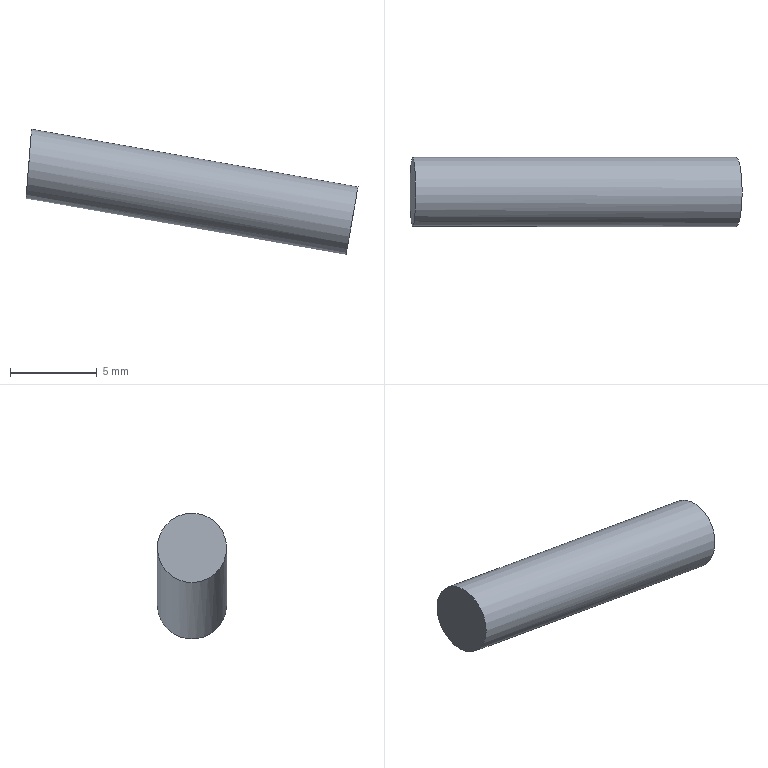Part | NX | features solid 2 | 1 solid | 3 faces | box 19.165 x 4 x 7.262 mm | volume 238.067 mm3 | plane 2 | cylinder 1 | commonest cylinder face diameters 4 x1
STEP:
#1=CARTESIAN_POINT('',(-434.591,688.216,-41.881));
#2=VERTEX_POINT('',#1);
#3=CARTESIAN_POINT('',(-434.591,686.216,-41.881));
#4=DIRECTION('',(-0.9848,0.,0.1736));
#5=DIRECTION('',(0.,1.,0.));
#6=AXIS2_PLACEMENT_3D('',#3,#4,#5);
#7=CIRCLE('',#6,2.);
#8=EDGE_CURVE('',#2,#2,#7,.T.);
#9=ORIENTED_EDGE('',*,*,#8,.T.);
#10=EDGE_LOOP('',(#9));
#11=FACE_BOUND('',#10,.T.);
#12=CARTESIAN_POINT('',(-453.408,686.216,-40.593));
#13=VERTEX_POINT('',#12);
#14=CARTESIAN_POINT('',(-453.248,686.216,-38.591));
#15=DIRECTION('',(-0.9968,0.,0.08003));
#16=DIRECTION('',(-0.08003,0.,-0.9968));
#17=AXIS2_PLACEMENT_3D('',#14,#15,#16);
#18=ELLIPSE('',#17,2.009,2.);
#19=EDGE_CURVE('',#13,#13,#18,.T.);
#20=ORIENTED_EDGE('',*,*,#19,.F.);
#21=EDGE_LOOP('',(#20));
#22=FACE_BOUND('',#21,.T.);
#23=CARTESIAN_POINT('',(-454.287,686.216,-38.408));
#24=DIRECTION('',(0.9848,0.,-0.1736));
#25=DIRECTION('',(0.1736,0.,0.9848));
#26=AXIS2_PLACEMENT_3D('',#23,#24,#25);
#27=CYLINDRICAL_SURFACE('',#26,2.);
#28=ADVANCED_FACE('',(#11,#22),#27,.T.);
#29=ORIENTED_EDGE('',*,*,#8,.F.);
#30=EDGE_LOOP('',(#29));
#31=FACE_BOUND('',#30,.T.);
#32=CARTESIAN_POINT('',(-434.591,686.216,-41.881));
#33=DIRECTION('',(-0.9848,0.,0.1736));
#34=DIRECTION('',(-0.1736,0.,-0.9848));
#35=AXIS2_PLACEMENT_3D('',#32,#33,#34);
#36=PLANE('',#35);
#37=ADVANCED_FACE('',(#31),#36,.F.);
#38=ORIENTED_EDGE('',*,*,#19,.T.);
#39=EDGE_LOOP('',(#38));
#40=FACE_BOUND('',#39,.T.);
#41=CARTESIAN_POINT('',(-448.537,482.597,20.085));
#42=DIRECTION('',(-0.9968,0.,0.08003));
#43=DIRECTION('',(-0.08003,0.,-0.9968));
#44=AXIS2_PLACEMENT_3D('',#41,#42,#43);
#45=PLANE('',#44);
#46=ADVANCED_FACE('',(#40),#45,.T.);
#47=CLOSED_SHELL('',(#28,#37,#46));
#48=MANIFOLD_SOLID_BREP('',#47);
#49=(LENGTH_UNIT()NAMED_UNIT(*)SI_UNIT(.MILLI.,.METRE.));
#50=UNCERTAINTY_MEASURE_WITH_UNIT(LENGTH_MEASURE(0.00001),#49,'','');
#51=(NAMED_UNIT(*)PLANE_ANGLE_UNIT()SI_UNIT($,.RADIAN.));
#52=(NAMED_UNIT(*)SI_UNIT($,.STERADIAN.)SOLID_ANGLE_UNIT());
#53=(GEOMETRIC_REPRESENTATION_CONTEXT(3)GLOBAL_UNCERTAINTY_ASSIGNED_CONTEXT((#50))GLOBAL_UNIT_ASSIGNED_CONTEXT((#49,#51,#52))REPRESENTATION_CONTEXT('',''));
#54=ADVANCED_BREP_SHAPE_REPRESENTATION('',(#48),#53);